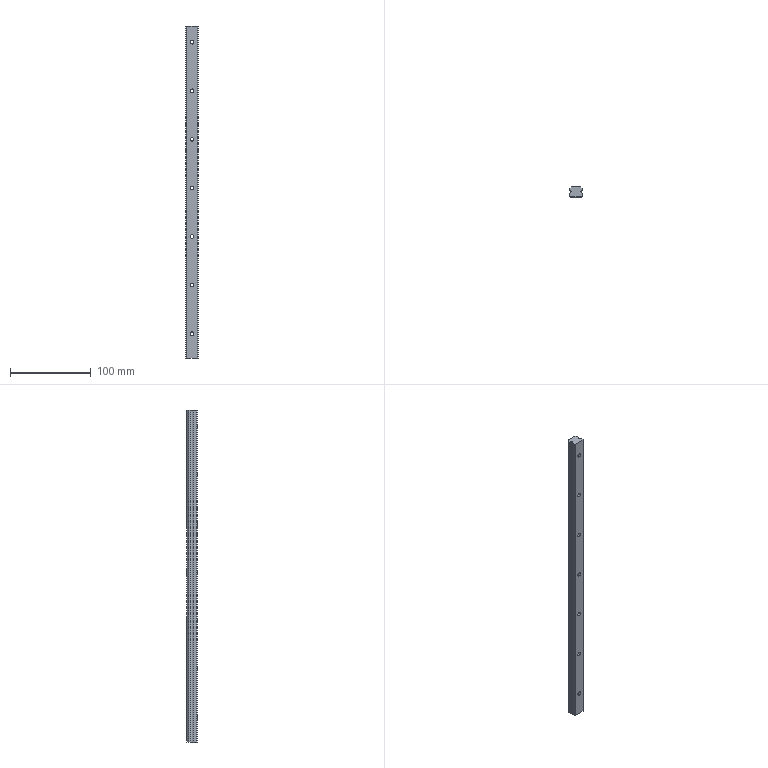Part | STEP file | MHC-H24-2-L410 Shanglong guide rail | 1 solid | 86 faces | box 15 x 12.5 x 410 mm | volume 68741 mm3 | cylinder 35 | cone 28 | plane 23 | commonest cylinder face diameters 4.5 x14 7.5 x14 3.5 x4 0.7 x3